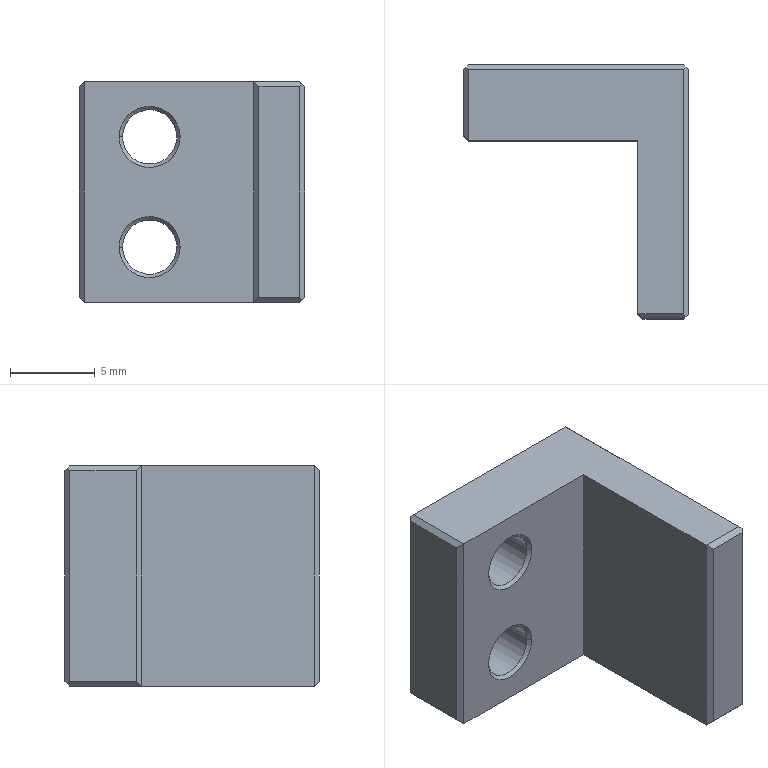Part | NX | 1 solid | 29 faces | box 13.3 x 15 x 13 mm | volume 1109 mm3 | plane 21 | cylinder 4 | cone 4 | commonest cylinder face diameters 3.2 x4
STEP:
#1=CARTESIAN_POINT('',(-175.3,172.2,-82.3));
#2=VERTEX_POINT('',#1);
#3=CARTESIAN_POINT('',(-177.7,172.2,-82.3));
#4=VERTEX_POINT('',#3);
#5=CARTESIAN_POINT('',(-176.5,172.2,-82.3));
#6=DIRECTION('',(-1.,0.,0.));
#7=VECTOR('',#6,1000.);
#8=LINE('',#5,#7);
#9=EDGE_CURVE('',#2,#4,#8,.T.);
#10=ORIENTED_EDGE('',*,*,#9,.T.);
#11=CARTESIAN_POINT('',(-177.7,172.2,-94.7));
#12=VERTEX_POINT('',#11);
#13=CARTESIAN_POINT('',(-177.7,172.2,-88.5));
#14=DIRECTION('',(0.,0.,1.));
#15=VECTOR('',#14,1000.);
#16=LINE('',#13,#15);
#17=EDGE_CURVE('',#12,#4,#16,.T.);
#18=ORIENTED_EDGE('',*,*,#17,.F.);
#19=CARTESIAN_POINT('',(-175.3,172.2,-94.7));
#20=VERTEX_POINT('',#19);
#21=CARTESIAN_POINT('',(-176.5,172.2,-94.7));
#22=DIRECTION('',(-1.,0.,0.));
#23=VECTOR('',#22,1000.);
#24=LINE('',#21,#23);
#25=EDGE_CURVE('',#20,#12,#24,.T.);
#26=ORIENTED_EDGE('',*,*,#25,.F.);
#27=CARTESIAN_POINT('',(-175.3,172.2,-88.5));
#28=DIRECTION('',(0.,0.,1.));
#29=VECTOR('',#28,1000.);
#30=LINE('',#27,#29);
#31=EDGE_CURVE('',#20,#2,#30,.T.);
#32=ORIENTED_EDGE('',*,*,#31,.T.);
#33=EDGE_LOOP('',(#10,#18,#26,#32));
#34=FACE_BOUND('',#33,.T.);
#35=CARTESIAN_POINT('',(-175.,172.2,-82.));
#36=DIRECTION('',(0.,-1.,0.));
#37=DIRECTION('',(-1.,0.,0.));
#38=AXIS2_PLACEMENT_3D('',#35,#36,#37);
#39=PLANE('',#38);
#40=ADVANCED_FACE('',(#34),#39,.T.);
#41=CARTESIAN_POINT('',(-188.,187.2,-94.7));
#42=VERTEX_POINT('',#41);
#43=CARTESIAN_POINT('',(-188.,187.2,-82.3));
#44=VERTEX_POINT('',#43);
#45=CARTESIAN_POINT('',(-188.,187.2,-88.5));
#46=DIRECTION('',(0.,0.,1.));
#47=VECTOR('',#46,1000.);
#48=LINE('',#45,#47);
#49=EDGE_CURVE('',#42,#44,#48,.T.);
#50=ORIENTED_EDGE('',*,*,#49,.T.);
#51=CARTESIAN_POINT('',(-175.3,187.2,-82.3));
#52=VERTEX_POINT('',#51);
#53=CARTESIAN_POINT('',(-175.,187.2,-82.3));
#54=DIRECTION('',(-1.,0.,0.));
#55=VECTOR('',#54,1000.);
#56=LINE('',#53,#55);
#57=EDGE_CURVE('',#52,#44,#56,.T.);
#58=ORIENTED_EDGE('',*,*,#57,.F.);
#59=CARTESIAN_POINT('',(-175.3,187.2,-94.7));
#60=VERTEX_POINT('',#59);
#61=CARTESIAN_POINT('',(-175.3,187.2,-88.5));
#62=DIRECTION('',(0.,0.,-1.));
#63=VECTOR('',#62,1000.);
#64=LINE('',#61,#63);
#65=EDGE_CURVE('',#52,#60,#64,.T.);
#66=ORIENTED_EDGE('',*,*,#65,.T.);
#67=CARTESIAN_POINT('',(-175.,187.2,-94.7));
#68=DIRECTION('',(-1.,0.,0.));
#69=VECTOR('',#68,1000.);
#70=LINE('',#67,#69);
#71=EDGE_CURVE('',#60,#42,#70,.T.);
#72=ORIENTED_EDGE('',*,*,#71,.T.);
#73=EDGE_LOOP('',(#50,#58,#66,#72));
#74=FACE_BOUND('',#73,.T.);
#75=CARTESIAN_POINT('',(-185.75,187.2,-91.75));
#76=VERTEX_POINT('',#75);
#77=CARTESIAN_POINT('',(-182.55,187.2,-91.75));
#78=VERTEX_POINT('',#77);
#79=CARTESIAN_POINT('',(-184.15,187.2,-91.75));
#80=DIRECTION('',(0.,-1.,0.));
#81=DIRECTION('',(1.,0.,0.));
#82=AXIS2_PLACEMENT_3D('',#79,#80,#81);
#83=CIRCLE('',#82,1.6);
#84=EDGE_CURVE('',#76,#78,#83,.T.);
#85=ORIENTED_EDGE('',*,*,#84,.T.);
#86=CARTESIAN_POINT('',(-184.15,187.2,-91.75));
#87=DIRECTION('',(0.,-1.,0.));
#88=DIRECTION('',(1.,0.,0.));
#89=AXIS2_PLACEMENT_3D('',#86,#87,#88);
#90=CIRCLE('',#89,1.6);
#91=EDGE_CURVE('',#78,#76,#90,.T.);
#92=ORIENTED_EDGE('',*,*,#91,.T.);
#93=EDGE_LOOP('',(#85,#92));
#94=FACE_BOUND('',#93,.T.);
#95=CARTESIAN_POINT('',(-185.75,187.2,-85.25));
#96=VERTEX_POINT('',#95);
#97=CARTESIAN_POINT('',(-182.55,187.2,-85.25));
#98=VERTEX_POINT('',#97);
#99=CARTESIAN_POINT('',(-184.15,187.2,-85.25));
#100=DIRECTION('',(0.,-1.,0.));
#101=DIRECTION('',(1.,0.,0.));
#102=AXIS2_PLACEMENT_3D('',#99,#100,#101);
#103=CIRCLE('',#102,1.6);
#104=EDGE_CURVE('',#96,#98,#103,.T.);
#105=ORIENTED_EDGE('',*,*,#104,.T.);
#106=CARTESIAN_POINT('',(-184.15,187.2,-85.25));
#107=DIRECTION('',(0.,-1.,0.));
#108=DIRECTION('',(1.,0.,0.));
#109=AXIS2_PLACEMENT_3D('',#106,#107,#108);
#110=CIRCLE('',#109,1.6);
#111=EDGE_CURVE('',#98,#96,#110,.T.);
#112=ORIENTED_EDGE('',*,*,#111,.T.);
#113=EDGE_LOOP('',(#105,#112));
#114=FACE_BOUND('',#113,.T.);
#115=CARTESIAN_POINT('',(-190.3,187.2,-95.944));
#116=DIRECTION('',(0.,1.,0.));
#117=DIRECTION('',(0.,0.,-1.));
#118=AXIS2_PLACEMENT_3D('',#115,#116,#117);
#119=PLANE('',#118);
#120=ADVANCED_FACE('',(#74,#94,#114),#119,.T.);
#121=CARTESIAN_POINT('',(-188.3,186.9,-94.7));
#122=VERTEX_POINT('',#121);
#123=CARTESIAN_POINT('',(-188.3,186.9,-82.3));
#124=VERTEX_POINT('',#123);
#125=CARTESIAN_POINT('',(-188.3,186.9,-88.5));
#126=DIRECTION('',(0.,0.,1.));
#127=VECTOR('',#126,1000.);
#128=LINE('',#125,#127);
#129=EDGE_CURVE('',#122,#124,#128,.T.);
#130=ORIENTED_EDGE('',*,*,#129,.F.);
#131=CARTESIAN_POINT('',(-188.3,183.,-94.7));
#132=VERTEX_POINT('',#131);
#133=CARTESIAN_POINT('',(-188.3,184.8,-94.7));
#134=DIRECTION('',(0.,1.,0.));
#135=VECTOR('',#134,1000.);
#136=LINE('',#133,#135);
#137=EDGE_CURVE('',#132,#122,#136,.T.);
#138=ORIENTED_EDGE('',*,*,#137,.F.);
#139=CARTESIAN_POINT('',(-188.3,183.,-82.3));
#140=VERTEX_POINT('',#139);
#141=CARTESIAN_POINT('',(-188.3,183.,-88.5));
#142=DIRECTION('',(0.,0.,-1.));
#143=VECTOR('',#142,1000.);
#144=LINE('',#141,#143);
#145=EDGE_CURVE('',#140,#132,#144,.T.);
#146=ORIENTED_EDGE('',*,*,#145,.F.);
#147=CARTESIAN_POINT('',(-188.3,184.8,-82.3));
#148=DIRECTION('',(0.,1.,0.));
#149=VECTOR('',#148,1000.);
#150=LINE('',#147,#149);
#151=EDGE_CURVE('',#140,#124,#150,.T.);
#152=ORIENTED_EDGE('',*,*,#151,.T.);
#153=EDGE_LOOP('',(#130,#138,#146,#152));
#154=FACE_BOUND('',#153,.T.);
#155=CARTESIAN_POINT('',(-188.3,182.7,-95.944));
#156=DIRECTION('',(-1.,0.,0.));
#157=DIRECTION('',(0.,1.,0.));
#158=AXIS2_PLACEMENT_3D('',#155,#156,#157);
#159=PLANE('',#158);
#160=ADVANCED_FACE('',(#154),#159,.T.);
#161=CARTESIAN_POINT('',(-188.,182.7,-95.));
#162=VERTEX_POINT('',#161);
#163=CARTESIAN_POINT('',(-188.,186.9,-95.));
#164=VERTEX_POINT('',#163);
#165=CARTESIAN_POINT('',(-188.,184.8,-95.));
#166=DIRECTION('',(0.,1.,0.));
#167=VECTOR('',#166,1000.);
#168=LINE('',#165,#167);
#169=EDGE_CURVE('',#162,#164,#168,.T.);
#170=ORIENTED_EDGE('',*,*,#169,.T.);
#171=CARTESIAN_POINT('',(-175.3,186.9,-95.));
#172=VERTEX_POINT('',#171);
#173=CARTESIAN_POINT('',(-175.,186.9,-95.));
#174=DIRECTION('',(-1.,0.,0.));
#175=VECTOR('',#174,1000.);
#176=LINE('',#173,#175);
#177=EDGE_CURVE('',#172,#164,#176,.T.);
#178=ORIENTED_EDGE('',*,*,#177,.F.);
#179=CARTESIAN_POINT('',(-175.3,172.5,-95.));
#180=VERTEX_POINT('',#179);
#181=CARTESIAN_POINT('',(-175.3,179.7,-95.));
#182=DIRECTION('',(0.,-1.,0.));
#183=VECTOR('',#182,1000.);
#184=LINE('',#181,#183);
#185=EDGE_CURVE('',#172,#180,#184,.T.);
#186=ORIENTED_EDGE('',*,*,#185,.T.);
#187=CARTESIAN_POINT('',(-178.,172.5,-95.));
#188=VERTEX_POINT('',#187);
#189=CARTESIAN_POINT('',(-176.5,172.5,-95.));
#190=DIRECTION('',(-1.,0.,0.));
#191=VECTOR('',#190,1000.);
#192=LINE('',#189,#191);
#193=EDGE_CURVE('',#180,#188,#192,.T.);
#194=ORIENTED_EDGE('',*,*,#193,.T.);
#195=CARTESIAN_POINT('',(-178.,182.7,-95.));
#196=VERTEX_POINT('',#195);
#197=CARTESIAN_POINT('',(-178.,180.866,-95.));
#198=DIRECTION('',(0.,-1.,0.));
#199=VECTOR('',#198,1000.);
#200=LINE('',#197,#199);
#201=EDGE_CURVE('',#196,#188,#200,.T.);
#202=ORIENTED_EDGE('',*,*,#201,.F.);
#203=CARTESIAN_POINT('',(-175.,182.7,-95.));
#204=DIRECTION('',(1.,0.,0.));
#205=VECTOR('',#204,1000.);
#206=LINE('',#203,#205);
#207=EDGE_CURVE('',#162,#196,#206,.T.);
#208=ORIENTED_EDGE('',*,*,#207,.F.);
#209=EDGE_LOOP('',(#170,#178,#186,#194,#202,#208));
#210=FACE_BOUND('',#209,.T.);
#211=CARTESIAN_POINT('',(-176.432,184.505,-95.));
#212=DIRECTION('',(0.,0.,-1.));
#213=DIRECTION('',(-1.,0.,0.));
#214=AXIS2_PLACEMENT_3D('',#211,#212,#213);
#215=PLANE('',#214);
#216=ADVANCED_FACE('',(#210),#215,.T.);
#217=ORIENTED_EDGE('',*,*,#207,.T.);
#218=CARTESIAN_POINT('',(-178.,182.7,-82.));
#219=VERTEX_POINT('',#218);
#220=CARTESIAN_POINT('',(-178.,182.7,-87.033));
#221=DIRECTION('',(0.,0.,1.));
#222=VECTOR('',#221,1000.);
#223=LINE('',#220,#222);
#224=EDGE_CURVE('',#196,#219,#223,.T.);
#225=ORIENTED_EDGE('',*,*,#224,.T.);
#226=CARTESIAN_POINT('',(-188.,182.7,-82.));
#227=VERTEX_POINT('',#226);
#228=CARTESIAN_POINT('',(-175.,182.7,-82.));
#229=DIRECTION('',(1.,0.,0.));
#230=VECTOR('',#229,1000.);
#231=LINE('',#228,#230);
#232=EDGE_CURVE('',#227,#219,#231,.T.);
#233=ORIENTED_EDGE('',*,*,#232,.F.);
#234=CARTESIAN_POINT('',(-188.,182.7,-88.5));
#235=DIRECTION('',(0.,0.,-1.));
#236=VECTOR('',#235,1000.);
#237=LINE('',#234,#236);
#238=EDGE_CURVE('',#227,#162,#237,.T.);
#239=ORIENTED_EDGE('',*,*,#238,.T.);
#240=EDGE_LOOP('',(#217,#225,#233,#239));
#241=FACE_BOUND('',#240,.T.);
#242=CARTESIAN_POINT('',(-185.95,182.7,-91.75));
#243=VERTEX_POINT('',#242);
#244=CARTESIAN_POINT('',(-182.35,182.7,-91.75));
#245=VERTEX_POINT('',#244);
#246=CARTESIAN_POINT('',(-184.15,182.7,-91.75));
#247=DIRECTION('',(0.,-1.,0.));
#248=DIRECTION('',(1.,0.,0.));
#249=AXIS2_PLACEMENT_3D('',#246,#247,#248);
#250=CIRCLE('',#249,1.8);
#251=EDGE_CURVE('',#243,#245,#250,.T.);
#252=ORIENTED_EDGE('',*,*,#251,.F.);
#253=CARTESIAN_POINT('',(-184.15,182.7,-91.75));
#254=DIRECTION('',(0.,-1.,0.));
#255=DIRECTION('',(1.,0.,0.));
#256=AXIS2_PLACEMENT_3D('',#253,#254,#255);
#257=CIRCLE('',#256,1.8);
#258=EDGE_CURVE('',#245,#243,#257,.T.);
#259=ORIENTED_EDGE('',*,*,#258,.F.);
#260=EDGE_LOOP('',(#252,#259));
#261=FACE_BOUND('',#260,.T.);
#262=CARTESIAN_POINT('',(-185.95,182.7,-85.25));
#263=VERTEX_POINT('',#262);
#264=CARTESIAN_POINT('',(-182.35,182.7,-85.25));
#265=VERTEX_POINT('',#264);
#266=CARTESIAN_POINT('',(-184.15,182.7,-85.25));
#267=DIRECTION('',(0.,-1.,0.));
#268=DIRECTION('',(1.,0.,0.));
#269=AXIS2_PLACEMENT_3D('',#266,#267,#268);
#270=CIRCLE('',#269,1.8);
#271=EDGE_CURVE('',#263,#265,#270,.T.);
#272=ORIENTED_EDGE('',*,*,#271,.F.);
#273=CARTESIAN_POINT('',(-184.15,182.7,-85.25));
#274=DIRECTION('',(0.,-1.,0.));
#275=DIRECTION('',(1.,0.,0.));
#276=AXIS2_PLACEMENT_3D('',#273,#274,#275);
#277=CIRCLE('',#276,1.8);
#278=EDGE_CURVE('',#265,#263,#277,.T.);
#279=ORIENTED_EDGE('',*,*,#278,.F.);
#280=EDGE_LOOP('',(#272,#279));
#281=FACE_BOUND('',#280,.T.);
#282=CARTESIAN_POINT('',(-178.,182.7,-95.944));
#283=DIRECTION('',(0.,-1.,0.));
#284=DIRECTION('',(0.,0.,-1.));
#285=AXIS2_PLACEMENT_3D('',#282,#283,#284);
#286=PLANE('',#285);
#287=ADVANCED_FACE('',(#241,#261,#281),#286,.T.);
#288=CARTESIAN_POINT('',(-188.,186.9,-82.));
#289=VERTEX_POINT('',#288);
#290=CARTESIAN_POINT('',(-188.,184.8,-82.));
#291=DIRECTION('',(0.,1.,0.));
#292=VECTOR('',#291,1000.);
#293=LINE('',#290,#292);
#294=EDGE_CURVE('',#227,#289,#293,.T.);
#295=ORIENTED_EDGE('',*,*,#294,.F.);
#296=ORIENTED_EDGE('',*,*,#232,.T.);
#297=CARTESIAN_POINT('',(-178.,172.5,-82.));
#298=VERTEX_POINT('',#297);
#299=CARTESIAN_POINT('',(-178.,180.866,-82.));
#300=DIRECTION('',(0.,-1.,0.));
#301=VECTOR('',#300,1000.);
#302=LINE('',#299,#301);
#303=EDGE_CURVE('',#219,#298,#302,.T.);
#304=ORIENTED_EDGE('',*,*,#303,.T.);
#305=CARTESIAN_POINT('',(-175.3,172.5,-82.));
#306=VERTEX_POINT('',#305);
#307=CARTESIAN_POINT('',(-176.5,172.5,-82.));
#308=DIRECTION('',(-1.,0.,0.));
#309=VECTOR('',#308,1000.);
#310=LINE('',#307,#309);
#311=EDGE_CURVE('',#306,#298,#310,.T.);
#312=ORIENTED_EDGE('',*,*,#311,.F.);
#313=CARTESIAN_POINT('',(-175.3,186.9,-82.));
#314=VERTEX_POINT('',#313);
#315=CARTESIAN_POINT('',(-175.3,179.7,-82.));
#316=DIRECTION('',(0.,-1.,0.));
#317=VECTOR('',#316,1000.);
#318=LINE('',#315,#317);
#319=EDGE_CURVE('',#314,#306,#318,.T.);
#320=ORIENTED_EDGE('',*,*,#319,.F.);
#321=CARTESIAN_POINT('',(-175.,186.9,-82.));
#322=DIRECTION('',(-1.,0.,0.));
#323=VECTOR('',#322,1000.);
#324=LINE('',#321,#323);
#325=EDGE_CURVE('',#314,#289,#324,.T.);
#326=ORIENTED_EDGE('',*,*,#325,.T.);
#327=EDGE_LOOP('',(#295,#296,#304,#312,#320,#326));
#328=FACE_BOUND('',#327,.T.);
#329=CARTESIAN_POINT('',(-176.432,184.505,-82.));
#330=DIRECTION('',(0.,0.,-1.));
#331=DIRECTION('',(-1.,0.,0.));
#332=AXIS2_PLACEMENT_3D('',#329,#330,#331);
#333=PLANE('',#332);
#334=ADVANCED_FACE('',(#328),#333,.F.);
#335=CARTESIAN_POINT('',(-185.75,182.9,-85.25));
#336=VERTEX_POINT('',#335);
#337=CARTESIAN_POINT('',(-182.55,182.9,-85.25));
#338=VERTEX_POINT('',#337);
#339=CARTESIAN_POINT('',(-184.15,182.9,-85.25));
#340=DIRECTION('',(0.,-1.,0.));
#341=DIRECTION('',(1.,0.,0.));
#342=AXIS2_PLACEMENT_3D('',#339,#340,#341);
#343=CIRCLE('',#342,1.6);
#344=EDGE_CURVE('',#336,#338,#343,.T.);
#345=ORIENTED_EDGE('',*,*,#344,.T.);
#346=CARTESIAN_POINT('',(-182.55,182.7,-85.25));
#347=DIRECTION('',(0.,-1.,0.));
#348=VECTOR('',#347,1000.);
#349=LINE('',#346,#348);
#350=EDGE_CURVE('',#98,#338,#349,.T.);
#351=ORIENTED_EDGE('',*,*,#350,.F.);
#352=ORIENTED_EDGE('',*,*,#104,.F.);
#353=CARTESIAN_POINT('',(-185.75,182.7,-85.25));
#354=DIRECTION('',(0.,-1.,0.));
#355=VECTOR('',#354,1000.);
#356=LINE('',#353,#355);
#357=EDGE_CURVE('',#96,#336,#356,.T.);
#358=ORIENTED_EDGE('',*,*,#357,.T.);
#359=EDGE_LOOP('',(#345,#351,#352,#358));
#360=FACE_BOUND('',#359,.T.);
#361=CARTESIAN_POINT('',(-184.15,182.7,-85.25));
#362=DIRECTION('',(0.,-1.,0.));
#363=DIRECTION('',(1.,0.,0.));
#364=AXIS2_PLACEMENT_3D('',#361,#362,#363);
#365=CYLINDRICAL_SURFACE('',#364,1.6);
#366=ADVANCED_FACE('',(#360),#365,.F.);
#367=ORIENTED_EDGE('',*,*,#344,.F.);
#368=CARTESIAN_POINT('',(-185.75,182.9,-85.25));
#369=DIRECTION('',(-0.7071,-0.7071,0.));
#370=VECTOR('',#369,1000.);
#371=LINE('',#368,#370);
#372=EDGE_CURVE('',#336,#263,#371,.T.);
#373=ORIENTED_EDGE('',*,*,#372,.T.);
#374=ORIENTED_EDGE('',*,*,#271,.T.);
#375=CARTESIAN_POINT('',(-182.55,182.9,-85.25));
#376=DIRECTION('',(0.7071,-0.7071,0.));
#377=VECTOR('',#376,1000.);
#378=LINE('',#375,#377);
#379=EDGE_CURVE('',#338,#265,#378,.T.);
#380=ORIENTED_EDGE('',*,*,#379,.F.);
#381=EDGE_LOOP('',(#367,#373,#374,#380));
#382=FACE_BOUND('',#381,.T.);
#383=CARTESIAN_POINT('',(-184.15,182.9,-85.25));
#384=DIRECTION('',(0.,-1.,0.));
#385=DIRECTION('',(1.,0.,0.));
#386=AXIS2_PLACEMENT_3D('',#383,#384,#385);
#387=CONICAL_SURFACE('',#386,1.6,0.7854);
#388=ADVANCED_FACE('',(#382),#387,.F.);
#389=CARTESIAN_POINT('',(-185.75,182.9,-91.75));
#390=VERTEX_POINT('',#389);
#391=CARTESIAN_POINT('',(-182.55,182.9,-91.75));
#392=VERTEX_POINT('',#391);
#393=CARTESIAN_POINT('',(-184.15,182.9,-91.75));
#394=DIRECTION('',(0.,-1.,0.));
#395=DIRECTION('',(1.,0.,0.));
#396=AXIS2_PLACEMENT_3D('',#393,#394,#395);
#397=CIRCLE('',#396,1.6);
#398=EDGE_CURVE('',#390,#392,#397,.T.);
#399=ORIENTED_EDGE('',*,*,#398,.T.);
#400=CARTESIAN_POINT('',(-182.55,182.7,-91.75));
#401=DIRECTION('',(0.,-1.,0.));
#402=VECTOR('',#401,1000.);
#403=LINE('',#400,#402);
#404=EDGE_CURVE('',#78,#392,#403,.T.);
#405=ORIENTED_EDGE('',*,*,#404,.F.);
#406=ORIENTED_EDGE('',*,*,#84,.F.);
#407=CARTESIAN_POINT('',(-185.75,182.7,-91.75));
#408=DIRECTION('',(0.,-1.,0.));
#409=VECTOR('',#408,1000.);
#410=LINE('',#407,#409);
#411=EDGE_CURVE('',#76,#390,#410,.T.);
#412=ORIENTED_EDGE('',*,*,#411,.T.);
#413=EDGE_LOOP('',(#399,#405,#406,#412));
#414=FACE_BOUND('',#413,.T.);
#415=CARTESIAN_POINT('',(-184.15,182.7,-91.75));
#416=DIRECTION('',(0.,-1.,0.));
#417=DIRECTION('',(1.,0.,0.));
#418=AXIS2_PLACEMENT_3D('',#415,#416,#417);
#419=CYLINDRICAL_SURFACE('',#418,1.6);
#420=ADVANCED_FACE('',(#414),#419,.F.);
#421=ORIENTED_EDGE('',*,*,#398,.F.);
#422=CARTESIAN_POINT('',(-185.75,182.9,-91.75));
#423=DIRECTION('',(-0.7071,-0.7071,0.));
#424=VECTOR('',#423,1000.);
#425=LINE('',#422,#424);
#426=EDGE_CURVE('',#390,#243,#425,.T.);
#427=ORIENTED_EDGE('',*,*,#426,.T.);
#428=ORIENTED_EDGE('',*,*,#251,.T.);
#429=CARTESIAN_POINT('',(-182.55,182.9,-91.75));
#430=DIRECTION('',(0.7071,-0.7071,0.));
#431=VECTOR('',#430,1000.);
#432=LINE('',#429,#431);
#433=EDGE_CURVE('',#392,#245,#432,.T.);
#434=ORIENTED_EDGE('',*,*,#433,.F.);
#435=EDGE_LOOP('',(#421,#427,#428,#434));
#436=FACE_BOUND('',#435,.T.);
#437=CARTESIAN_POINT('',(-184.15,182.9,-91.75));
#438=DIRECTION('',(0.,-1.,0.));
#439=DIRECTION('',(1.,0.,0.));
#440=AXIS2_PLACEMENT_3D('',#437,#438,#439);
#441=CONICAL_SURFACE('',#440,1.6,0.7854);
#442=ADVANCED_FACE('',(#436),#441,.F.);
#443=ORIENTED_EDGE('',*,*,#25,.T.);
#444=CARTESIAN_POINT('',(-186.366,180.866,-103.366));
#445=DIRECTION('',(-0.5774,0.5774,-0.5774));
#446=VECTOR('',#445,1000.);
#447=LINE('',#444,#446);
#448=EDGE_CURVE('',#12,#188,#447,.T.);
#449=ORIENTED_EDGE('',*,*,#448,.T.);
#450=ORIENTED_EDGE('',*,*,#193,.F.);
#451=CARTESIAN_POINT('',(-175.15,172.35,-94.85));
#452=VERTEX_POINT('',#451);
#453=CARTESIAN_POINT('',(-183.666,180.866,-103.366));
#454=DIRECTION('',(-0.5774,0.5774,-0.5774));
#455=VECTOR('',#454,1000.);
#456=LINE('',#453,#455);
#457=EDGE_CURVE('',#452,#180,#456,.T.);
#458=ORIENTED_EDGE('',*,*,#457,.F.);
#459=CARTESIAN_POINT('',(-166.634,180.866,-103.366));
#460=DIRECTION('',(0.5774,0.5774,-0.5774));
#461=VECTOR('',#460,1000.);
#462=LINE('',#459,#461);
#463=EDGE_CURVE('',#20,#452,#462,.T.);
#464=ORIENTED_EDGE('',*,*,#463,.F.);
#465=EDGE_LOOP('',(#443,#449,#450,#458,#464));
#466=FACE_BOUND('',#465,.T.);
#467=CARTESIAN_POINT('',(-176.5,172.35,-94.85));
#468=DIRECTION('',(0.,0.7071,0.7071));
#469=DIRECTION('',(1.,0.,0.));
#470=AXIS2_PLACEMENT_3D('',#467,#468,#469);
#471=PLANE('',#470);
#472=ADVANCED_FACE('',(#466),#471,.F.);
#473=ORIENTED_EDGE('',*,*,#177,.T.);
#474=CARTESIAN_POINT('',(-188.15,187.05,-94.85));
#475=VERTEX_POINT('',#474);
#476=CARTESIAN_POINT('',(-175.,173.9,-108.));
#477=DIRECTION('',(-0.5774,0.5774,0.5774));
#478=VECTOR('',#477,1000.);
#479=LINE('',#476,#478);
#480=EDGE_CURVE('',#164,#475,#479,.T.);
#481=ORIENTED_EDGE('',*,*,#480,.T.);
#482=CARTESIAN_POINT('',(-194.334,180.866,-101.034));
#483=DIRECTION('',(-0.5774,-0.5774,-0.5774));
#484=VECTOR('',#483,1000.);
#485=LINE('',#482,#484);
#486=EDGE_CURVE('',#42,#475,#485,.T.);
#487=ORIENTED_EDGE('',*,*,#486,.F.);
#488=ORIENTED_EDGE('',*,*,#71,.F.);
#489=CARTESIAN_POINT('',(-175.15,187.05,-94.85));
#490=VERTEX_POINT('',#489);
#491=CARTESIAN_POINT('',(-175.,186.9,-95.));
#492=DIRECTION('',(0.5774,-0.5774,-0.5774));
#493=VECTOR('',#492,1000.);
#494=LINE('',#491,#493);
#495=EDGE_CURVE('',#60,#490,#494,.T.);
#496=ORIENTED_EDGE('',*,*,#495,.T.);
#497=CARTESIAN_POINT('',(-181.334,180.866,-101.034));
#498=DIRECTION('',(0.5774,0.5774,0.5774));
#499=VECTOR('',#498,1000.);
#500=LINE('',#497,#499);
#501=EDGE_CURVE('',#172,#490,#500,.T.);
#502=ORIENTED_EDGE('',*,*,#501,.F.);
#503=EDGE_LOOP('',(#473,#481,#487,#488,#496,#502));
#504=FACE_BOUND('',#503,.T.);
#505=CARTESIAN_POINT('',(-182.65,187.05,-94.85));
#506=DIRECTION('',(0.,-0.7071,0.7071));
#507=DIRECTION('',(-1.,0.,0.));
#508=AXIS2_PLACEMENT_3D('',#505,#506,#507);
#509=PLANE('',#508);
#510=ADVANCED_FACE('',(#504),#509,.F.);
#511=ORIENTED_EDGE('',*,*,#57,.T.);
#512=CARTESIAN_POINT('',(-188.15,187.05,-82.15));
#513=VERTEX_POINT('',#512);
#514=CARTESIAN_POINT('',(-183.267,191.933,-87.033));
#515=DIRECTION('',(-0.5773,-0.5773,0.5774));
#516=VECTOR('',#515,1000.);
#517=LINE('',#514,#516);
#518=EDGE_CURVE('',#44,#513,#517,.T.);
#519=ORIENTED_EDGE('',*,*,#518,.T.);
#520=CARTESIAN_POINT('',(-175.,173.9,-69.));
#521=DIRECTION('',(0.5774,-0.5773,0.5774));
#522=VECTOR('',#521,1000.);
#523=LINE('',#520,#522);
#524=EDGE_CURVE('',#513,#289,#523,.T.);
#525=ORIENTED_EDGE('',*,*,#524,.T.);
#526=ORIENTED_EDGE('',*,*,#325,.F.);
#527=CARTESIAN_POINT('',(-175.15,187.05,-82.15));
#528=VERTEX_POINT('',#527);
#529=CARTESIAN_POINT('',(-175.,187.2,-82.3));
#530=DIRECTION('',(0.5774,0.5773,-0.5774));
#531=VECTOR('',#530,1000.);
#532=LINE('',#529,#531);
#533=EDGE_CURVE('',#314,#528,#532,.T.);
#534=ORIENTED_EDGE('',*,*,#533,.T.);
#535=CARTESIAN_POINT('',(-180.033,191.933,-87.033));
#536=DIRECTION('',(0.5773,-0.5773,0.5774));
#537=VECTOR('',#536,1000.);
#538=LINE('',#535,#537);
#539=EDGE_CURVE('',#52,#528,#538,.T.);
#540=ORIENTED_EDGE('',*,*,#539,.F.);
#541=EDGE_LOOP('',(#511,#519,#525,#526,#534,#540));
#542=FACE_BOUND('',#541,.T.);
#543=CARTESIAN_POINT('',(-182.65,187.05,-82.15));
#544=DIRECTION('',(0.,0.7071,0.7071));
#545=DIRECTION('',(1.,0.,0.));
#546=AXIS2_PLACEMENT_3D('',#543,#544,#545);
#547=PLANE('',#546);
#548=ADVANCED_FACE('',(#542),#547,.T.);
#549=ORIENTED_EDGE('',*,*,#9,.F.);
#550=CARTESIAN_POINT('',(-175.15,172.35,-82.15));
#551=VERTEX_POINT('',#550);
#552=CARTESIAN_POINT('',(-166.634,180.866,-73.634));
#553=DIRECTION('',(0.5774,0.5774,0.5774));
#554=VECTOR('',#553,1000.);
#555=LINE('',#552,#554);
#556=EDGE_CURVE('',#2,#551,#555,.T.);
#557=ORIENTED_EDGE('',*,*,#556,.T.);
#558=CARTESIAN_POINT('',(-183.666,180.866,-73.634));
#559=DIRECTION('',(-0.5774,0.5774,0.5774));
#560=VECTOR('',#559,1000.);
#561=LINE('',#558,#560);
#562=EDGE_CURVE('',#551,#306,#561,.T.);
#563=ORIENTED_EDGE('',*,*,#562,.T.);
#564=ORIENTED_EDGE('',*,*,#311,.T.);
#565=CARTESIAN_POINT('',(-186.366,180.866,-73.634));
#566=DIRECTION('',(-0.5774,0.5774,0.5774));
#567=VECTOR('',#566,1000.);
#568=LINE('',#565,#567);
#569=EDGE_CURVE('',#4,#298,#568,.T.);
#570=ORIENTED_EDGE('',*,*,#569,.F.);
#571=EDGE_LOOP('',(#549,#557,#563,#564,#570));
#572=FACE_BOUND('',#571,.T.);
#573=CARTESIAN_POINT('',(-176.5,172.35,-82.15));
#574=DIRECTION('',(0.,-0.7071,0.7071));
#575=DIRECTION('',(-1.,0.,0.));
#576=AXIS2_PLACEMENT_3D('',#573,#574,#575);
#577=PLANE('',#576);
#578=ADVANCED_FACE('',(#572),#577,.T.);
#579=ORIENTED_EDGE('',*,*,#145,.T.);
#580=CARTESIAN_POINT('',(-175.,169.7,-108.));
#581=DIRECTION('',(-0.5774,0.5774,0.5774));
#582=VECTOR('',#581,1000.);
#583=LINE('',#580,#582);
#584=EDGE_CURVE('',#162,#132,#583,.T.);
#585=ORIENTED_EDGE('',*,*,#584,.F.);
#586=ORIENTED_EDGE('',*,*,#238,.F.);
#587=CARTESIAN_POINT('',(-175.,169.7,-69.));
#588=DIRECTION('',(-0.5774,0.5774,-0.5774));
#589=VECTOR('',#588,1000.);
#590=LINE('',#587,#589);
#591=EDGE_CURVE('',#227,#140,#590,.T.);
#592=ORIENTED_EDGE('',*,*,#591,.T.);
#593=EDGE_LOOP('',(#579,#585,#586,#592));
#594=FACE_BOUND('',#593,.T.);
#595=CARTESIAN_POINT('',(-188.15,182.85,-88.5));
#596=DIRECTION('',(0.7071,0.7071,0.));
#597=DIRECTION('',(0.,0.,-1.));
#598=AXIS2_PLACEMENT_3D('',#595,#596,#597);
#599=PLANE('',#598);
#600=ADVANCED_FACE('',(#594),#599,.F.);
#601=ORIENTED_EDGE('',*,*,#169,.F.);
#602=ORIENTED_EDGE('',*,*,#584,.T.);
#603=ORIENTED_EDGE('',*,*,#137,.T.);
#604=CARTESIAN_POINT('',(-194.334,180.866,-88.666));
#605=DIRECTION('',(0.5774,0.5774,-0.5774));
#606=VECTOR('',#605,1000.);
#607=LINE('',#604,#606);
#608=EDGE_CURVE('',#122,#475,#607,.T.);
#609=ORIENTED_EDGE('',*,*,#608,.T.);
#610=ORIENTED_EDGE('',*,*,#480,.F.);
#611=EDGE_LOOP('',(#601,#602,#603,#609,#610));
#612=FACE_BOUND('',#611,.T.);
#613=CARTESIAN_POINT('',(-188.15,184.8,-94.85));
#614=DIRECTION('',(-0.7071,0.,-0.7071));
#615=DIRECTION('',(-0.7071,0.,0.7071));
#616=AXIS2_PLACEMENT_3D('',#613,#614,#615);
#617=PLANE('',#616);
#618=ADVANCED_FACE('',(#612),#617,.T.);
#619=ORIENTED_EDGE('',*,*,#129,.T.);
#620=CARTESIAN_POINT('',(-194.334,180.866,-88.334));
#621=DIRECTION('',(-0.5774,-0.5774,-0.5774));
#622=VECTOR('',#621,1000.);
#623=LINE('',#620,#622);
#624=EDGE_CURVE('',#513,#124,#623,.T.);
#625=ORIENTED_EDGE('',*,*,#624,.F.);
#626=ORIENTED_EDGE('',*,*,#518,.F.);
#627=ORIENTED_EDGE('',*,*,#49,.F.);
#628=ORIENTED_EDGE('',*,*,#486,.T.);
#629=ORIENTED_EDGE('',*,*,#608,.F.);
#630=EDGE_LOOP('',(#619,#625,#626,#627,#628,#629));
#631=FACE_BOUND('',#630,.T.);
#632=CARTESIAN_POINT('',(-188.15,187.05,-88.5));
#633=DIRECTION('',(0.7071,-0.7071,0.));
#634=DIRECTION('',(0.,0.,-1.));
#635=AXIS2_PLACEMENT_3D('',#632,#633,#634);
#636=PLANE('',#635);
#637=ADVANCED_FACE('',(#631),#636,.F.);
#638=ORIENTED_EDGE('',*,*,#294,.T.);
#639=ORIENTED_EDGE('',*,*,#524,.F.);
#640=ORIENTED_EDGE('',*,*,#624,.T.);
#641=ORIENTED_EDGE('',*,*,#151,.F.);
#642=ORIENTED_EDGE('',*,*,#591,.F.);
#643=EDGE_LOOP('',(#638,#639,#640,#641,#642));
#644=FACE_BOUND('',#643,.T.);
#645=CARTESIAN_POINT('',(-188.15,184.8,-82.15));
#646=DIRECTION('',(0.7071,0.,-0.7071));
#647=DIRECTION('',(0.,-1.,0.));
#648=AXIS2_PLACEMENT_3D('',#645,#646,#647);
#649=PLANE('',#648);
#650=ADVANCED_FACE('',(#644),#649,.F.);
#651=ORIENTED_EDGE('',*,*,#404,.T.);
#652=CARTESIAN_POINT('',(-184.15,182.9,-91.75));
#653=DIRECTION('',(0.,-1.,0.));
#654=DIRECTION('',(1.,0.,0.));
#655=AXIS2_PLACEMENT_3D('',#652,#653,#654);
#656=CIRCLE('',#655,1.6);
#657=EDGE_CURVE('',#392,#390,#656,.T.);
#658=ORIENTED_EDGE('',*,*,#657,.T.);
#659=ORIENTED_EDGE('',*,*,#411,.F.);
#660=ORIENTED_EDGE('',*,*,#91,.F.);
#661=EDGE_LOOP('',(#651,#658,#659,#660));
#662=FACE_BOUND('',#661,.T.);
#663=CARTESIAN_POINT('',(-184.15,182.7,-91.75));
#664=DIRECTION('',(0.,-1.,0.));
#665=DIRECTION('',(1.,0.,0.));
#666=AXIS2_PLACEMENT_3D('',#663,#664,#665);
#667=CYLINDRICAL_SURFACE('',#666,1.6);
#668=ADVANCED_FACE('',(#662),#667,.F.);
#669=ORIENTED_EDGE('',*,*,#433,.T.);
#670=ORIENTED_EDGE('',*,*,#258,.T.);
#671=ORIENTED_EDGE('',*,*,#426,.F.);
#672=ORIENTED_EDGE('',*,*,#657,.F.);
#673=EDGE_LOOP('',(#669,#670,#671,#672));
#674=FACE_BOUND('',#673,.T.);
#675=CARTESIAN_POINT('',(-184.15,182.9,-91.75));
#676=DIRECTION('',(0.,-1.,0.));
#677=DIRECTION('',(1.,0.,0.));
#678=AXIS2_PLACEMENT_3D('',#675,#676,#677);
#679=CONICAL_SURFACE('',#678,1.6,0.7854);
#680=ADVANCED_FACE('',(#674),#679,.F.);
#681=ORIENTED_EDGE('',*,*,#350,.T.);
#682=CARTESIAN_POINT('',(-184.15,182.9,-85.25));
#683=DIRECTION('',(0.,-1.,0.));
#684=DIRECTION('',(1.,0.,0.));
#685=AXIS2_PLACEMENT_3D('',#682,#683,#684);
#686=CIRCLE('',#685,1.6);
#687=EDGE_CURVE('',#338,#336,#686,.T.);
#688=ORIENTED_EDGE('',*,*,#687,.T.);
#689=ORIENTED_EDGE('',*,*,#357,.F.);
#690=ORIENTED_EDGE('',*,*,#111,.F.);
#691=EDGE_LOOP('',(#681,#688,#689,#690));
#692=FACE_BOUND('',#691,.T.);
#693=CARTESIAN_POINT('',(-184.15,182.7,-85.25));
#694=DIRECTION('',(0.,-1.,0.));
#695=DIRECTION('',(1.,0.,0.));
#696=AXIS2_PLACEMENT_3D('',#693,#694,#695);
#697=CYLINDRICAL_SURFACE('',#696,1.6);
#698=ADVANCED_FACE('',(#692),#697,.F.);
#699=ORIENTED_EDGE('',*,*,#379,.T.);
#700=ORIENTED_EDGE('',*,*,#278,.T.);
#701=ORIENTED_EDGE('',*,*,#372,.F.);
#702=ORIENTED_EDGE('',*,*,#687,.F.);
#703=EDGE_LOOP('',(#699,#700,#701,#702));
#704=FACE_BOUND('',#703,.T.);
#705=CARTESIAN_POINT('',(-184.15,182.9,-85.25));
#706=DIRECTION('',(0.,-1.,0.));
#707=DIRECTION('',(1.,0.,0.));
#708=AXIS2_PLACEMENT_3D('',#705,#706,#707);
#709=CONICAL_SURFACE('',#708,1.6,0.7854);
#710=ADVANCED_FACE('',(#704),#709,.F.);
#711=CARTESIAN_POINT('',(-178.,172.5,-88.5));
#712=DIRECTION('',(0.,0.,1.));
#713=VECTOR('',#712,1000.);
#714=LINE('',#711,#713);
#715=EDGE_CURVE('',#188,#298,#714,.T.);
#716=ORIENTED_EDGE('',*,*,#715,.T.);
#717=ORIENTED_EDGE('',*,*,#303,.F.);
#718=ORIENTED_EDGE('',*,*,#224,.F.);
#719=ORIENTED_EDGE('',*,*,#201,.T.);
#720=EDGE_LOOP('',(#716,#717,#718,#719));
#721=FACE_BOUND('',#720,.T.);
#722=CARTESIAN_POINT('',(-178.,180.866,-87.033));
#723=DIRECTION('',(-1.,0.,0.));
#724=DIRECTION('',(0.,0.,1.));
#725=AXIS2_PLACEMENT_3D('',#722,#723,#724);
#726=PLANE('',#725);
#727=ADVANCED_FACE('',(#721),#726,.T.);
#728=ORIENTED_EDGE('',*,*,#715,.F.);
#729=ORIENTED_EDGE('',*,*,#448,.F.);
#730=ORIENTED_EDGE('',*,*,#17,.T.);
#731=ORIENTED_EDGE('',*,*,#569,.T.);
#732=EDGE_LOOP('',(#728,#729,#730,#731));
#733=FACE_BOUND('',#732,.T.);
#734=CARTESIAN_POINT('',(-177.85,172.35,-88.5));
#735=DIRECTION('',(-0.7071,-0.7071,0.));
#736=DIRECTION('',(-0.7071,0.7071,0.));
#737=AXIS2_PLACEMENT_3D('',#734,#735,#736);
#738=PLANE('',#737);
#739=ADVANCED_FACE('',(#733),#738,.T.);
#740=CARTESIAN_POINT('',(-175.,186.9,-82.3));
#741=VERTEX_POINT('',#740);
#742=CARTESIAN_POINT('',(-175.,172.5,-82.3));
#743=VERTEX_POINT('',#742);
#744=CARTESIAN_POINT('',(-175.,179.7,-82.3));
#745=DIRECTION('',(0.,-1.,0.));
#746=VECTOR('',#745,1000.);
#747=LINE('',#744,#746);
#748=EDGE_CURVE('',#741,#743,#747,.T.);
#749=ORIENTED_EDGE('',*,*,#748,.T.);
#750=CARTESIAN_POINT('',(-175.,172.5,-94.7));
#751=VERTEX_POINT('',#750);
#752=CARTESIAN_POINT('',(-175.,172.5,-88.5));
#753=DIRECTION('',(0.,0.,1.));
#754=VECTOR('',#753,1000.);
#755=LINE('',#752,#754);
#756=EDGE_CURVE('',#751,#743,#755,.T.);
#757=ORIENTED_EDGE('',*,*,#756,.F.);
#758=CARTESIAN_POINT('',(-175.,186.9,-94.7));
#759=VERTEX_POINT('',#758);
#760=CARTESIAN_POINT('',(-175.,179.7,-94.7));
#761=DIRECTION('',(0.,-1.,0.));
#762=VECTOR('',#761,1000.);
#763=LINE('',#760,#762);
#764=EDGE_CURVE('',#759,#751,#763,.T.);
#765=ORIENTED_EDGE('',*,*,#764,.F.);
#766=CARTESIAN_POINT('',(-175.,186.9,-88.5));
#767=DIRECTION('',(0.,0.,-1.));
#768=VECTOR('',#767,1000.);
#769=LINE('',#766,#768);
#770=EDGE_CURVE('',#741,#759,#769,.T.);
#771=ORIENTED_EDGE('',*,*,#770,.F.);
#772=EDGE_LOOP('',(#749,#757,#765,#771));
#773=FACE_BOUND('',#772,.T.);
#774=CARTESIAN_POINT('',(-175.,180.866,-87.033));
#775=DIRECTION('',(-1.,0.,0.));
#776=DIRECTION('',(0.,0.,1.));
#777=AXIS2_PLACEMENT_3D('',#774,#775,#776);
#778=PLANE('',#777);
#779=ADVANCED_FACE('',(#773),#778,.F.);
#780=ORIENTED_EDGE('',*,*,#764,.T.);
#781=CARTESIAN_POINT('',(-166.634,180.866,-86.334));
#782=DIRECTION('',(-0.5774,-0.5774,-0.5774));
#783=VECTOR('',#782,1000.);
#784=LINE('',#781,#783);
#785=EDGE_CURVE('',#751,#452,#784,.T.);
#786=ORIENTED_EDGE('',*,*,#785,.T.);
#787=ORIENTED_EDGE('',*,*,#457,.T.);
#788=ORIENTED_EDGE('',*,*,#185,.F.);
#789=ORIENTED_EDGE('',*,*,#501,.T.);
#790=CARTESIAN_POINT('',(-175.,186.9,-94.7));
#791=DIRECTION('',(0.5774,-0.5774,0.5774));
#792=VECTOR('',#791,1000.);
#793=LINE('',#790,#792);
#794=EDGE_CURVE('',#490,#759,#793,.T.);
#795=ORIENTED_EDGE('',*,*,#794,.T.);
#796=EDGE_LOOP('',(#780,#786,#787,#788,#789,#795));
#797=FACE_BOUND('',#796,.T.);
#798=CARTESIAN_POINT('',(-175.15,179.7,-94.85));
#799=DIRECTION('',(-0.7071,0.,0.7071));
#800=DIRECTION('',(0.,1.,0.));
#801=AXIS2_PLACEMENT_3D('',#798,#799,#800);
#802=PLANE('',#801);
#803=ADVANCED_FACE('',(#797),#802,.F.);
#804=ORIENTED_EDGE('',*,*,#756,.T.);
#805=CARTESIAN_POINT('',(-166.634,180.866,-90.666));
#806=DIRECTION('',(0.5774,0.5774,-0.5774));
#807=VECTOR('',#806,1000.);
#808=LINE('',#805,#807);
#809=EDGE_CURVE('',#551,#743,#808,.T.);
#810=ORIENTED_EDGE('',*,*,#809,.F.);
#811=ORIENTED_EDGE('',*,*,#556,.F.);
#812=ORIENTED_EDGE('',*,*,#31,.F.);
#813=ORIENTED_EDGE('',*,*,#463,.T.);
#814=ORIENTED_EDGE('',*,*,#785,.F.);
#815=EDGE_LOOP('',(#804,#810,#811,#812,#813,#814));
#816=FACE_BOUND('',#815,.T.);
#817=CARTESIAN_POINT('',(-175.15,172.35,-88.5));
#818=DIRECTION('',(-0.7071,0.7071,0.));
#819=DIRECTION('',(0.,0.,1.));
#820=AXIS2_PLACEMENT_3D('',#817,#818,#819);
#821=PLANE('',#820);
#822=ADVANCED_FACE('',(#816),#821,.F.);
#823=ORIENTED_EDGE('',*,*,#770,.T.);
#824=ORIENTED_EDGE('',*,*,#794,.F.);
#825=ORIENTED_EDGE('',*,*,#495,.F.);
#826=ORIENTED_EDGE('',*,*,#65,.F.);
#827=ORIENTED_EDGE('',*,*,#539,.T.);
#828=CARTESIAN_POINT('',(-175.,186.9,-82.3));
#829=DIRECTION('',(-0.5774,0.5774,0.5774));
#830=VECTOR('',#829,1000.);
#831=LINE('',#828,#830);
#832=EDGE_CURVE('',#741,#528,#831,.T.);
#833=ORIENTED_EDGE('',*,*,#832,.F.);
#834=EDGE_LOOP('',(#823,#824,#825,#826,#827,#833));
#835=FACE_BOUND('',#834,.T.);
#836=CARTESIAN_POINT('',(-175.15,187.05,-88.5));
#837=DIRECTION('',(-0.7071,-0.7071,0.));
#838=DIRECTION('',(-0.7071,0.7071,0.));
#839=AXIS2_PLACEMENT_3D('',#836,#837,#838);
#840=PLANE('',#839);
#841=ADVANCED_FACE('',(#835),#840,.F.);
#842=ORIENTED_EDGE('',*,*,#748,.F.);
#843=ORIENTED_EDGE('',*,*,#832,.T.);
#844=ORIENTED_EDGE('',*,*,#533,.F.);
#845=ORIENTED_EDGE('',*,*,#319,.T.);
#846=ORIENTED_EDGE('',*,*,#562,.F.);
#847=ORIENTED_EDGE('',*,*,#809,.T.);
#848=EDGE_LOOP('',(#842,#843,#844,#845,#846,#847));
#849=FACE_BOUND('',#848,.T.);
#850=CARTESIAN_POINT('',(-175.15,179.7,-82.15));
#851=DIRECTION('',(0.7071,0.,0.7071));
#852=DIRECTION('',(0.,-1.,0.));
#853=AXIS2_PLACEMENT_3D('',#850,#851,#852);
#854=PLANE('',#853);
#855=ADVANCED_FACE('',(#849),#854,.T.);
#856=CLOSED_SHELL('',(#40,#120,#160,#216,#287,#334,#366,#388,#420,#442,#472,#510,#548,#578,#600,#618,#637,#650,#668,#680,#698,#710,#727,#739,#779,#803,#822,#841,#855));
#857=MANIFOLD_SOLID_BREP('',#856);
#858=(LENGTH_UNIT()NAMED_UNIT(*)SI_UNIT(.MILLI.,.METRE.));
#859=UNCERTAINTY_MEASURE_WITH_UNIT(LENGTH_MEASURE(0.00001),#858,'','');
#860=(NAMED_UNIT(*)PLANE_ANGLE_UNIT()SI_UNIT($,.RADIAN.));
#861=(NAMED_UNIT(*)SI_UNIT($,.STERADIAN.)SOLID_ANGLE_UNIT());
#862=(GEOMETRIC_REPRESENTATION_CONTEXT(3)GLOBAL_UNCERTAINTY_ASSIGNED_CONTEXT((#859))GLOBAL_UNIT_ASSIGNED_CONTEXT((#858,#860,#861))REPRESENTATION_CONTEXT('',''));
#863=ADVANCED_BREP_SHAPE_REPRESENTATION('',(#857),#862);